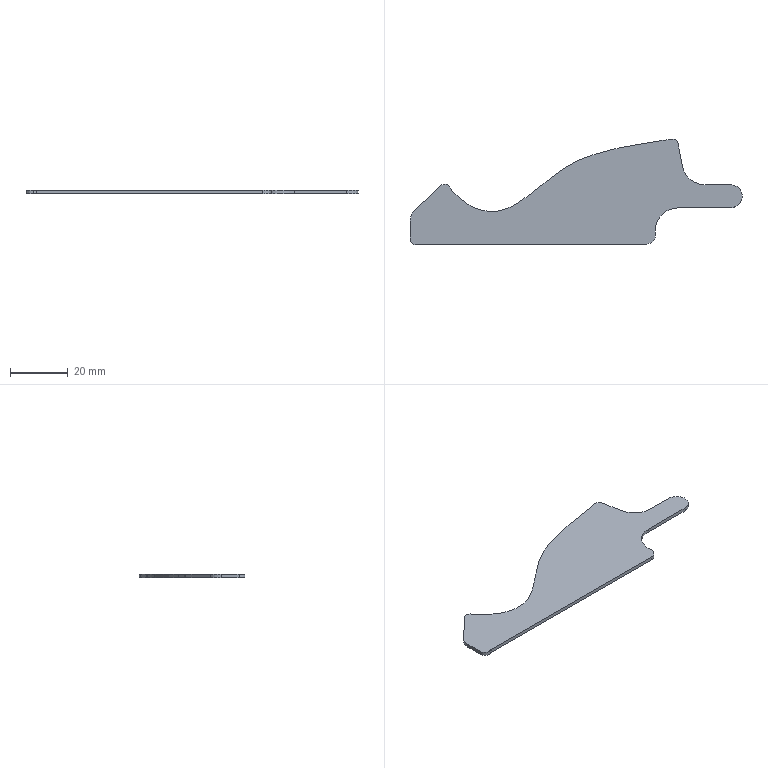Part | STEP file | gslz 2016.10.28-13_id162_x_t | 1 solid | 32 faces | box 114.754 x 36.538 x 1.25 mm | volume 2820 mm3 | plane 19 | cylinder 13 | commonest cylinder face diameters 4 x5 16 x2 6 x1 8 x1 10 x1 30 x1